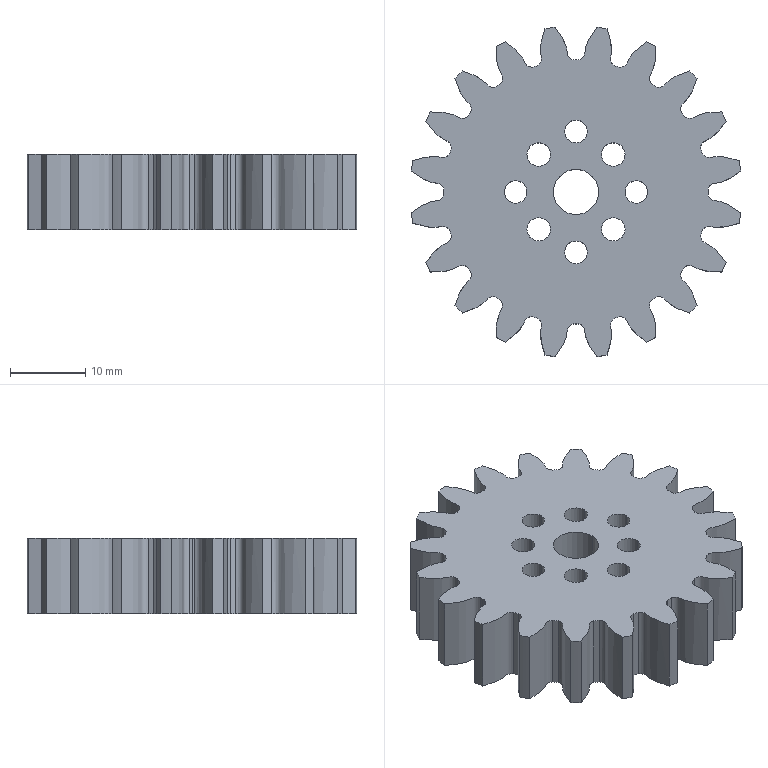Part | STEP file | FD gear 20 | 1 solid | 104 faces | box 43.654 x 43.654 x 10 mm | volume 10262 mm3 | cylinder 61 | spline 40 | plane 3 | commonest cylinder face diameters 35 x21 44 x20 3 x8 3.1 x8 6 x2 25 x2